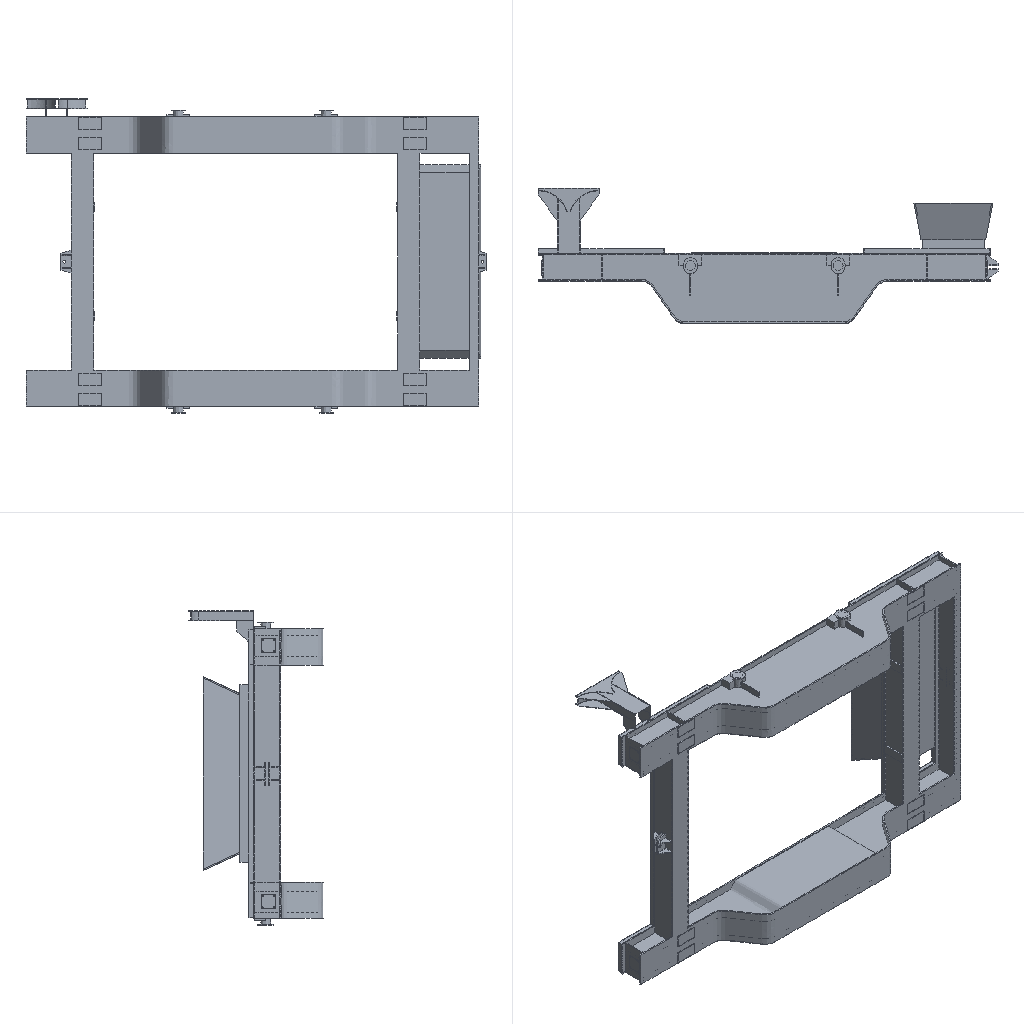Simulation study | ansys workbench
Set-up summary:
category,name,step,type,value,unit,region
solver,ansys_mapdl
solver,version,,,22.1
solver,version,,,22.1
units,MPA,,stated
analysis,deck1,,static,static
load_step,requested,,,1
analysis,nlgeom,,,False
mesh,nodes,,,29872
mesh,elements,,,31502
element_type,ANSYS 181 (type 1),,shell,30433
element_type,ANSYS 154 (type 2),,surface,1069
load,load commands in deck,,count,3
bc,support commands in deck,,count,1
named_set,_FIXEDSU,,component
analysis,deck2,,static,static
load_step,requested,,,1
analysis,nlgeom,,,False
mesh,nodes,,,29872
mesh,elements,,,33735
element_type,ANSYS 181 (type 1),,shell,30433
element_type,ANSYS 154 (type 2),,surface,3302
load,load commands in deck,,count,3
bc,support commands in deck,,count,1
named_set,_FIXEDSU,,component
material,1,,in results
material,1,,in results
check,setup vs results,,match,1069 surface effect element(s) are not in the reader's mesh and were not compared
check,setup vs results,,match,3302 surface effect element(s) are not in the reader's mesh and were not compared
Results summary:
result,analysis,,,static
result,last_loadstep,,,1
result,primary field,,,displacement
result,reaction total,1,FX,-1e-06,N
result,reaction total,1,FY,500.0,N
result,reaction total,1,FZ,-0.0,N
result,mass,,,0.1314,"NMM: mm, ton, N, s, mV, mA, degC"
result,analysis,,,static
result,last_loadstep,,,1
result,primary field,,,displacement
result,reaction total,1,FX,-1e-06,N
result,reaction total,1,FY,500.0,N
result,reaction total,1,FZ,1e-06,N
result,mass,,,0.1314,"NMM: mm, ton, N, s, mV, mA, degC"